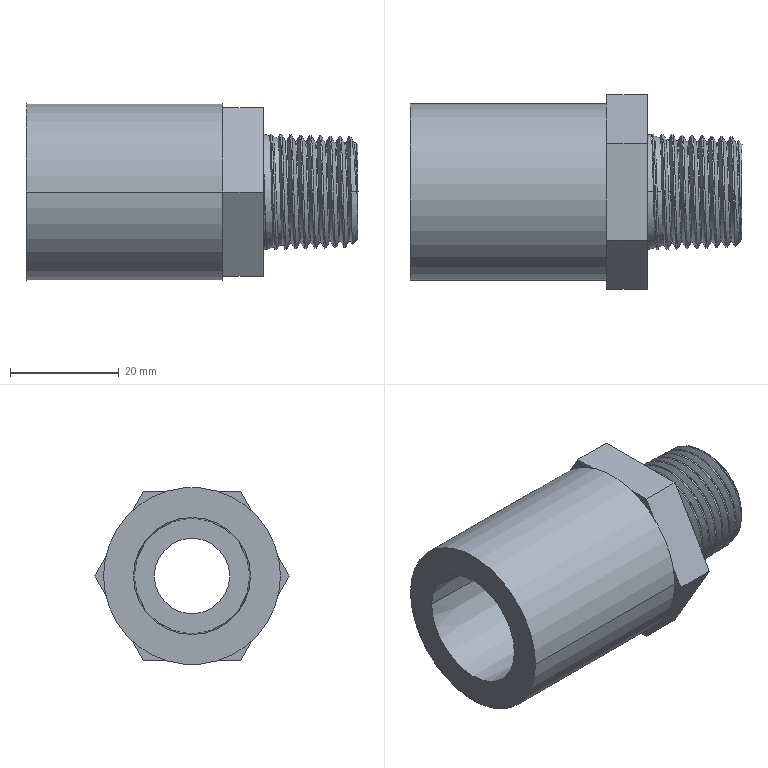Part | SolidWorks | features BaseBody 2 | 2 solids | 52 faces | box 61.119 x 35.745 x 32.544 mm | volume 27815 mm3 | cone 31 | plane 12 | cylinder 6 | spline 3 | commonest cylinder face diameters 13.868 x4 32.544 x2